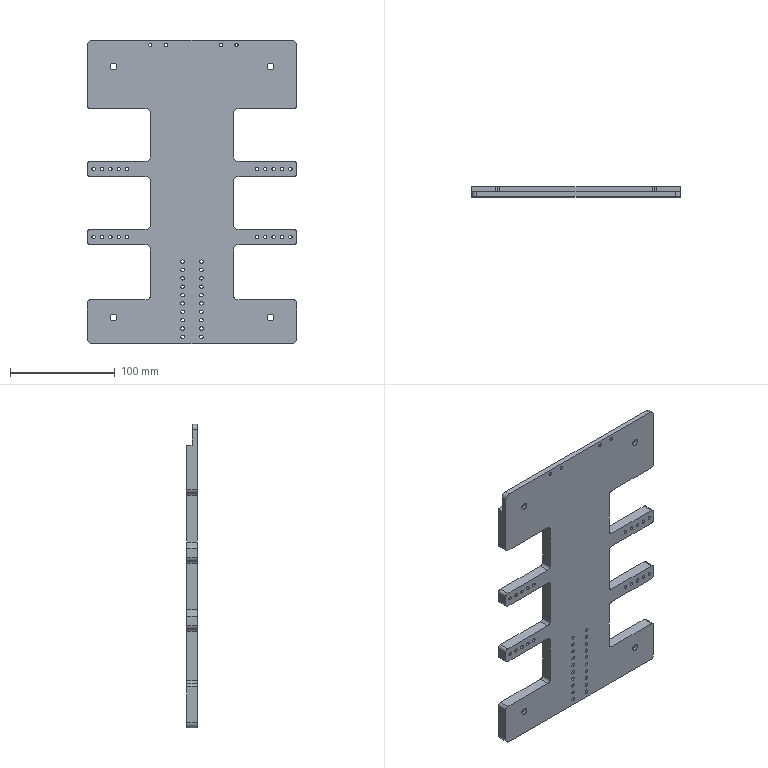Part | STEP file | 0-19-09 Discharge platform | 1 solid | 170 faces | box 200 x 10 x 290 mm | volume 370239 mm3 | cylinder 132 | plane 38 | commonest cylinder face diameters 3.3 x88 6 x24 6.6 x8 11 x8 10 x4